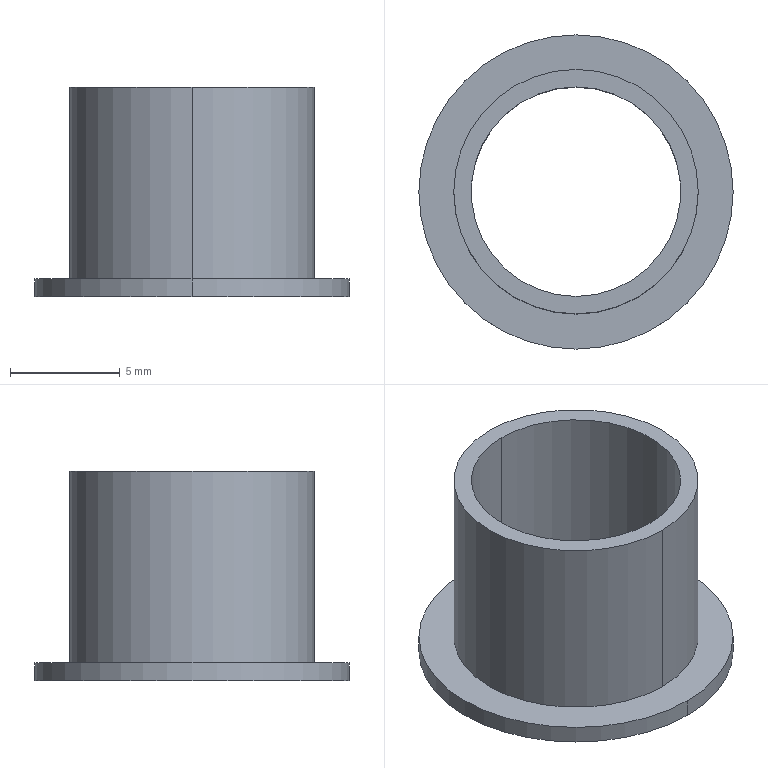Part | NX | features BREP 1 | 1 solid | 9 faces | box 14.287 x 14.287 x 9.525 mm | volume 296.572 mm3 | cylinder 6 | plane 3 | commonest cylinder face diameters 9.525 x2 11.113 x2 14.287 x2
STEP:
#1=CARTESIAN_POINT('',(0.,4.763,9.525));
#2=VERTEX_POINT('',#1);
#3=CARTESIAN_POINT('',(0.,-4.763,9.525));
#4=VERTEX_POINT('',#3);
#5=CARTESIAN_POINT('',(0.,0.,9.525));
#6=DIRECTION('',(0.,0.,1.));
#7=DIRECTION('',(0.,1.,0.));
#8=AXIS2_PLACEMENT_3D('',#5,#6,#7);
#9=CIRCLE('',#8,4.763);
#10=EDGE_CURVE('',#2,#4,#9,.T.);
#11=ORIENTED_EDGE('',*,*,#10,.T.);
#12=CARTESIAN_POINT('',(0.,-4.763,0.));
#13=VERTEX_POINT('',#12);
#14=CARTESIAN_POINT('',(0.,-4.763,0.));
#15=DIRECTION('',(0.,0.,1.));
#16=VECTOR('',#15,1000.);
#17=LINE('',#14,#16);
#18=EDGE_CURVE('',#4,#13,#17,.F.);
#19=ORIENTED_EDGE('',*,*,#18,.T.);
#20=CARTESIAN_POINT('',(0.,4.763,0.));
#21=VERTEX_POINT('',#20);
#22=CARTESIAN_POINT('',(0.,0.,0.));
#23=DIRECTION('',(0.,0.,1.));
#24=DIRECTION('',(0.,1.,0.));
#25=AXIS2_PLACEMENT_3D('',#22,#23,#24);
#26=CIRCLE('',#25,4.763);
#27=EDGE_CURVE('',#21,#13,#26,.T.);
#28=ORIENTED_EDGE('',*,*,#27,.F.);
#29=CARTESIAN_POINT('',(0.,4.763,0.));
#30=DIRECTION('',(0.,0.,1.));
#31=VECTOR('',#30,1000.);
#32=LINE('',#29,#31);
#33=EDGE_CURVE('',#2,#21,#32,.F.);
#34=ORIENTED_EDGE('',*,*,#33,.F.);
#35=EDGE_LOOP('',(#11,#19,#28,#34));
#36=FACE_BOUND('',#35,.T.);
#37=CARTESIAN_POINT('',(0.,0.,-0.4763));
#38=DIRECTION('',(0.,0.,1.));
#39=DIRECTION('',(0.,-1.,0.));
#40=AXIS2_PLACEMENT_3D('',#37,#38,#39);
#41=CYLINDRICAL_SURFACE('',#40,4.763);
#42=ADVANCED_FACE('',(#36),#41,.F.);
#43=CARTESIAN_POINT('',(0.,0.,0.));
#44=DIRECTION('',(0.,0.,-1.));
#45=DIRECTION('',(0.,1.,0.));
#46=AXIS2_PLACEMENT_3D('',#43,#44,#45);
#47=CIRCLE('',#46,4.763);
#48=EDGE_CURVE('',#21,#13,#47,.T.);
#49=ORIENTED_EDGE('',*,*,#48,.T.);
#50=ORIENTED_EDGE('',*,*,#18,.F.);
#51=CARTESIAN_POINT('',(0.,0.,9.525));
#52=DIRECTION('',(0.,0.,-1.));
#53=DIRECTION('',(0.,1.,0.));
#54=AXIS2_PLACEMENT_3D('',#51,#52,#53);
#55=CIRCLE('',#54,4.763);
#56=EDGE_CURVE('',#2,#4,#55,.T.);
#57=ORIENTED_EDGE('',*,*,#56,.F.);
#58=ORIENTED_EDGE('',*,*,#33,.T.);
#59=EDGE_LOOP('',(#49,#50,#57,#58));
#60=FACE_BOUND('',#59,.T.);
#61=CARTESIAN_POINT('',(0.,0.,-0.4763));
#62=DIRECTION('',(0.,0.,1.));
#63=DIRECTION('',(0.,-1.,0.));
#64=AXIS2_PLACEMENT_3D('',#61,#62,#63);
#65=CYLINDRICAL_SURFACE('',#64,4.763);
#66=ADVANCED_FACE('',(#60),#65,.F.);
#67=CARTESIAN_POINT('',(0.,5.556,9.525));
#68=VERTEX_POINT('',#67);
#69=CARTESIAN_POINT('',(0.,-5.556,9.525));
#70=VERTEX_POINT('',#69);
#71=CARTESIAN_POINT('',(0.,0.,9.525));
#72=DIRECTION('',(0.,0.,-1.));
#73=DIRECTION('',(0.,1.,0.));
#74=AXIS2_PLACEMENT_3D('',#71,#72,#73);
#75=CIRCLE('',#74,5.556);
#76=EDGE_CURVE('',#68,#70,#75,.T.);
#77=ORIENTED_EDGE('',*,*,#76,.F.);
#78=CARTESIAN_POINT('',(0.,0.,9.525));
#79=DIRECTION('',(0.,0.,1.));
#80=DIRECTION('',(0.,1.,0.));
#81=AXIS2_PLACEMENT_3D('',#78,#79,#80);
#82=CIRCLE('',#81,5.556);
#83=EDGE_CURVE('',#68,#70,#82,.T.);
#84=ORIENTED_EDGE('',*,*,#83,.T.);
#85=EDGE_LOOP('',(#77,#84));
#86=FACE_BOUND('',#85,.T.);
#87=ORIENTED_EDGE('',*,*,#10,.F.);
#88=ORIENTED_EDGE('',*,*,#56,.T.);
#89=EDGE_LOOP('',(#87,#88));
#90=FACE_BOUND('',#89,.T.);
#91=CARTESIAN_POINT('',(0.,0.,9.525));
#92=DIRECTION('',(0.,0.,1.));
#93=DIRECTION('',(1.,0.,0.));
#94=AXIS2_PLACEMENT_3D('',#91,#92,#93);
#95=PLANE('',#94);
#96=ADVANCED_FACE('',(#86,#90),#95,.T.);
#97=CARTESIAN_POINT('',(0.,5.556,0.8128));
#98=VERTEX_POINT('',#97);
#99=CARTESIAN_POINT('',(0.,-5.556,0.8128));
#100=VERTEX_POINT('',#99);
#101=CARTESIAN_POINT('',(0.,0.,0.8128));
#102=DIRECTION('',(0.,0.,1.));
#103=DIRECTION('',(0.,1.,0.));
#104=AXIS2_PLACEMENT_3D('',#101,#102,#103);
#105=CIRCLE('',#104,5.556);
#106=EDGE_CURVE('',#98,#100,#105,.T.);
#107=ORIENTED_EDGE('',*,*,#106,.T.);
#108=CARTESIAN_POINT('',(0.,-5.556,9.525));
#109=DIRECTION('',(0.,0.,-1.));
#110=VECTOR('',#109,1000.);
#111=LINE('',#108,#110);
#112=EDGE_CURVE('',#100,#70,#111,.F.);
#113=ORIENTED_EDGE('',*,*,#112,.T.);
#114=ORIENTED_EDGE('',*,*,#83,.F.);
#115=CARTESIAN_POINT('',(0.,5.556,9.525));
#116=DIRECTION('',(0.,0.,-1.));
#117=VECTOR('',#116,1000.);
#118=LINE('',#115,#117);
#119=EDGE_CURVE('',#98,#68,#118,.F.);
#120=ORIENTED_EDGE('',*,*,#119,.F.);
#121=EDGE_LOOP('',(#107,#113,#114,#120));
#122=FACE_BOUND('',#121,.T.);
#123=CARTESIAN_POINT('',(0.,0.,-0.4763));
#124=DIRECTION('',(0.,0.,1.));
#125=DIRECTION('',(0.,-1.,0.));
#126=AXIS2_PLACEMENT_3D('',#123,#124,#125);
#127=CYLINDRICAL_SURFACE('',#126,5.556);
#128=ADVANCED_FACE('',(#122),#127,.T.);
#129=ORIENTED_EDGE('',*,*,#76,.T.);
#130=ORIENTED_EDGE('',*,*,#112,.F.);
#131=CARTESIAN_POINT('',(0.,0.,0.8128));
#132=DIRECTION('',(0.,0.,-1.));
#133=DIRECTION('',(0.,1.,0.));
#134=AXIS2_PLACEMENT_3D('',#131,#132,#133);
#135=CIRCLE('',#134,5.556);
#136=EDGE_CURVE('',#98,#100,#135,.T.);
#137=ORIENTED_EDGE('',*,*,#136,.F.);
#138=ORIENTED_EDGE('',*,*,#119,.T.);
#139=EDGE_LOOP('',(#129,#130,#137,#138));
#140=FACE_BOUND('',#139,.T.);
#141=CARTESIAN_POINT('',(0.,0.,-0.4763));
#142=DIRECTION('',(0.,0.,1.));
#143=DIRECTION('',(0.,-1.,0.));
#144=AXIS2_PLACEMENT_3D('',#141,#142,#143);
#145=CYLINDRICAL_SURFACE('',#144,5.556);
#146=ADVANCED_FACE('',(#140),#145,.T.);
#147=CARTESIAN_POINT('',(0.,7.144,0.8128));
#148=VERTEX_POINT('',#147);
#149=CARTESIAN_POINT('',(0.,-7.144,0.8128));
#150=VERTEX_POINT('',#149);
#151=CARTESIAN_POINT('',(0.,0.,0.8128));
#152=DIRECTION('',(0.,0.,-1.));
#153=DIRECTION('',(0.,1.,0.));
#154=AXIS2_PLACEMENT_3D('',#151,#152,#153);
#155=CIRCLE('',#154,7.144);
#156=EDGE_CURVE('',#148,#150,#155,.T.);
#157=ORIENTED_EDGE('',*,*,#156,.F.);
#158=CARTESIAN_POINT('',(0.,0.,0.8128));
#159=DIRECTION('',(0.,0.,1.));
#160=DIRECTION('',(0.,1.,0.));
#161=AXIS2_PLACEMENT_3D('',#158,#159,#160);
#162=CIRCLE('',#161,7.144);
#163=EDGE_CURVE('',#148,#150,#162,.T.);
#164=ORIENTED_EDGE('',*,*,#163,.T.);
#165=EDGE_LOOP('',(#157,#164));
#166=FACE_BOUND('',#165,.T.);
#167=ORIENTED_EDGE('',*,*,#106,.F.);
#168=ORIENTED_EDGE('',*,*,#136,.T.);
#169=EDGE_LOOP('',(#167,#168));
#170=FACE_BOUND('',#169,.T.);
#171=CARTESIAN_POINT('',(0.,0.,0.8128));
#172=DIRECTION('',(0.,0.,1.));
#173=DIRECTION('',(1.,0.,0.));
#174=AXIS2_PLACEMENT_3D('',#171,#172,#173);
#175=PLANE('',#174);
#176=ADVANCED_FACE('',(#166,#170),#175,.T.);
#177=CARTESIAN_POINT('',(0.,7.144,0.));
#178=VERTEX_POINT('',#177);
#179=CARTESIAN_POINT('',(0.,-7.144,0.));
#180=VERTEX_POINT('',#179);
#181=CARTESIAN_POINT('',(0.,0.,0.));
#182=DIRECTION('',(0.,0.,1.));
#183=DIRECTION('',(0.,1.,0.));
#184=AXIS2_PLACEMENT_3D('',#181,#182,#183);
#185=CIRCLE('',#184,7.144);
#186=EDGE_CURVE('',#178,#180,#185,.T.);
#187=ORIENTED_EDGE('',*,*,#186,.T.);
#188=CARTESIAN_POINT('',(0.,-7.144,0.8128));
#189=DIRECTION('',(0.,0.,-1.));
#190=VECTOR('',#189,1000.);
#191=LINE('',#188,#190);
#192=EDGE_CURVE('',#180,#150,#191,.F.);
#193=ORIENTED_EDGE('',*,*,#192,.T.);
#194=ORIENTED_EDGE('',*,*,#163,.F.);
#195=CARTESIAN_POINT('',(0.,7.144,0.8128));
#196=DIRECTION('',(0.,0.,-1.));
#197=VECTOR('',#196,1000.);
#198=LINE('',#195,#197);
#199=EDGE_CURVE('',#178,#148,#198,.F.);
#200=ORIENTED_EDGE('',*,*,#199,.F.);
#201=EDGE_LOOP('',(#187,#193,#194,#200));
#202=FACE_BOUND('',#201,.T.);
#203=CARTESIAN_POINT('',(0.,0.,-0.4763));
#204=DIRECTION('',(0.,0.,1.));
#205=DIRECTION('',(0.,-1.,0.));
#206=AXIS2_PLACEMENT_3D('',#203,#204,#205);
#207=CYLINDRICAL_SURFACE('',#206,7.144);
#208=ADVANCED_FACE('',(#202),#207,.T.);
#209=ORIENTED_EDGE('',*,*,#156,.T.);
#210=ORIENTED_EDGE('',*,*,#192,.F.);
#211=CARTESIAN_POINT('',(0.,0.,0.));
#212=DIRECTION('',(0.,0.,-1.));
#213=DIRECTION('',(0.,1.,0.));
#214=AXIS2_PLACEMENT_3D('',#211,#212,#213);
#215=CIRCLE('',#214,7.144);
#216=EDGE_CURVE('',#178,#180,#215,.T.);
#217=ORIENTED_EDGE('',*,*,#216,.F.);
#218=ORIENTED_EDGE('',*,*,#199,.T.);
#219=EDGE_LOOP('',(#209,#210,#217,#218));
#220=FACE_BOUND('',#219,.T.);
#221=CARTESIAN_POINT('',(0.,0.,-0.4763));
#222=DIRECTION('',(0.,0.,1.));
#223=DIRECTION('',(0.,-1.,0.));
#224=AXIS2_PLACEMENT_3D('',#221,#222,#223);
#225=CYLINDRICAL_SURFACE('',#224,7.144);
#226=ADVANCED_FACE('',(#220),#225,.T.);
#227=ORIENTED_EDGE('',*,*,#186,.F.);
#228=ORIENTED_EDGE('',*,*,#216,.T.);
#229=EDGE_LOOP('',(#227,#228));
#230=FACE_BOUND('',#229,.T.);
#231=ORIENTED_EDGE('',*,*,#48,.F.);
#232=ORIENTED_EDGE('',*,*,#27,.T.);
#233=EDGE_LOOP('',(#231,#232));
#234=FACE_BOUND('',#233,.T.);
#235=CARTESIAN_POINT('',(0.,0.,0.));
#236=DIRECTION('',(0.,0.,1.));
#237=DIRECTION('',(1.,0.,0.));
#238=AXIS2_PLACEMENT_3D('',#235,#236,#237);
#239=PLANE('',#238);
#240=ADVANCED_FACE('',(#230,#234),#239,.F.);
#241=CLOSED_SHELL('',(#42,#66,#96,#128,#146,#176,#208,#226,#240));
#242=MANIFOLD_SOLID_BREP('',#241);
#243=(LENGTH_UNIT()NAMED_UNIT(*)SI_UNIT(.MILLI.,.METRE.));
#244=UNCERTAINTY_MEASURE_WITH_UNIT(LENGTH_MEASURE(0.00001),#243,'','');
#245=(NAMED_UNIT(*)PLANE_ANGLE_UNIT()SI_UNIT($,.RADIAN.));
#246=(NAMED_UNIT(*)SI_UNIT($,.STERADIAN.)SOLID_ANGLE_UNIT());
#247=(GEOMETRIC_REPRESENTATION_CONTEXT(3)GLOBAL_UNCERTAINTY_ASSIGNED_CONTEXT((#244))GLOBAL_UNIT_ASSIGNED_CONTEXT((#243,#245,#246))REPRESENTATION_CONTEXT('',''));
#248=ADVANCED_BREP_SHAPE_REPRESENTATION('',(#242),#247);